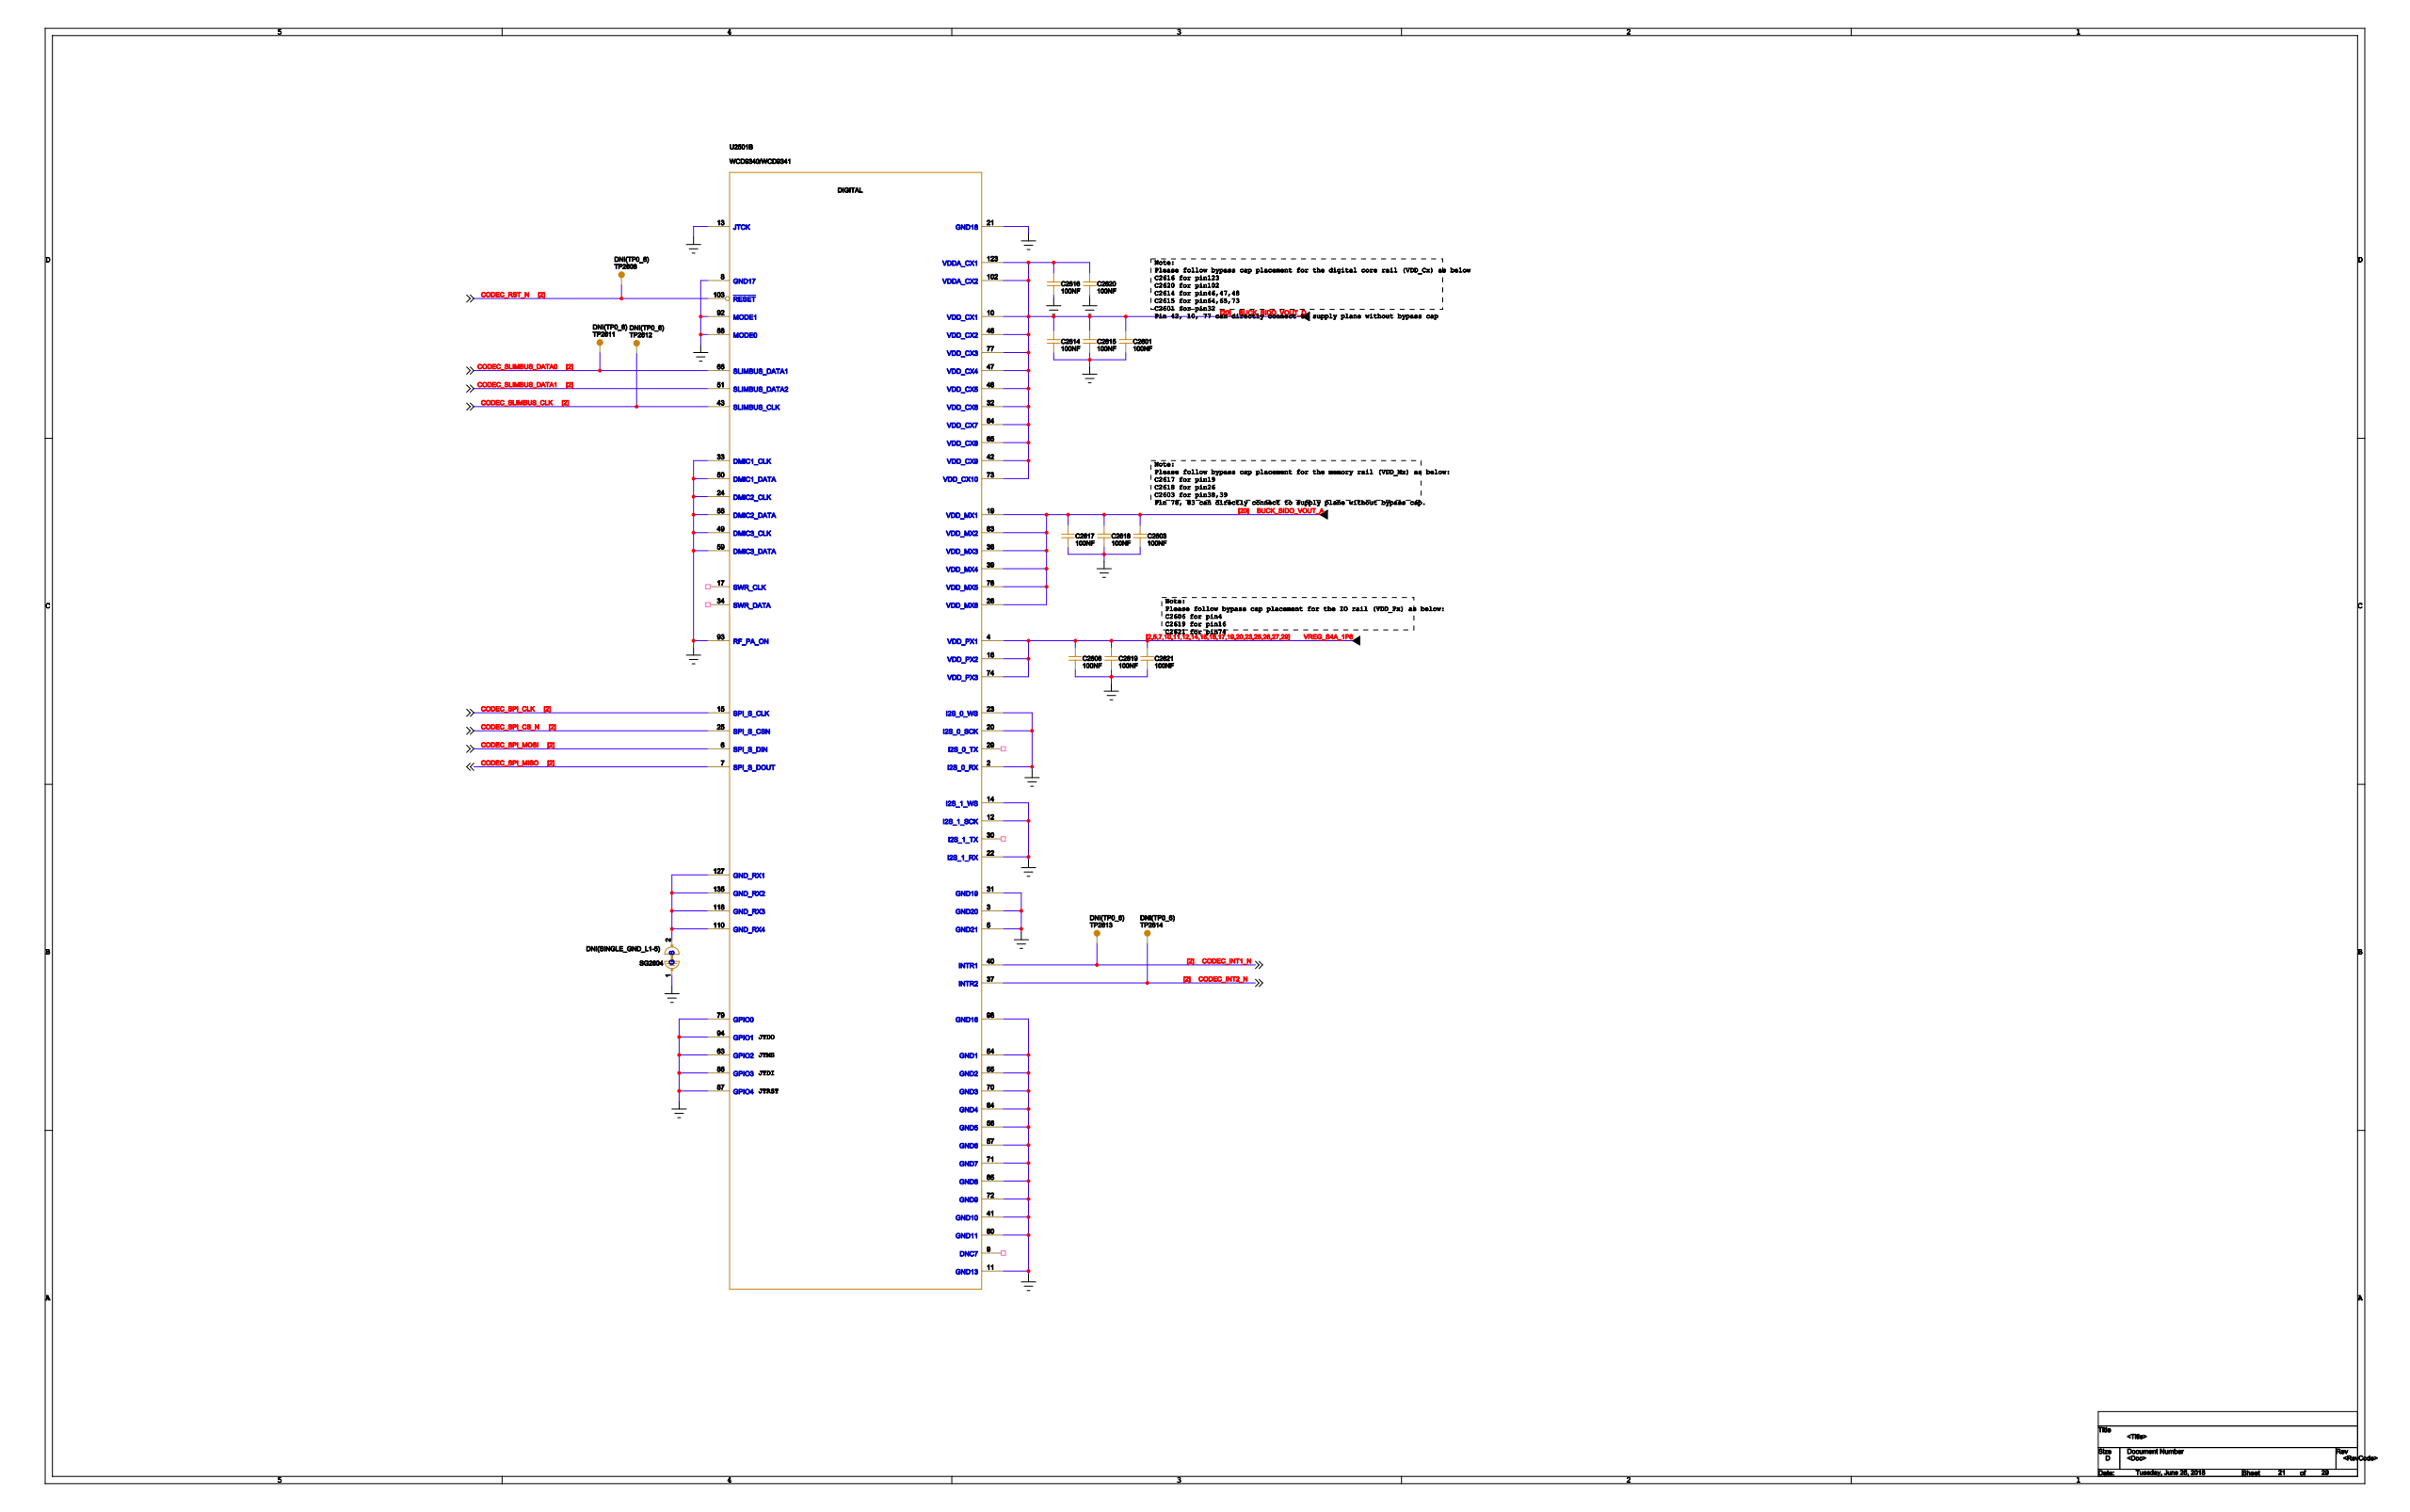Circuit board | Cadence Allegro | 802 parts | 566 nets | one sheet of the schematic
Parts on this sheet (reference | value | footprint):
C2601 | 100NF | C0201
C2603 | 100NF | C0201
C2606 | 100NF | C0201
C2614 | 100NF | C0201
C2615 | 100NF | C0201
C2616 | 100NF | C0201
C2617 | 100NF | C0201
C2618 | 100NF | C0201
C2619 | 100NF | C0201
C2620 | 100NF | C0201
C2621 | 100NF | C0201
SG2604 | DNI(SINGLE_GND_L1-5) | GND_L1-5
TP2608 | DNI(TP0_6) | TP_C0P6
TP2611 | DNI(TP0_6) | TP_C0P6
TP2612 | DNI(TP0_6) | TP_C0P6
TP2613 | DNI(TP0_6) | TP_C0P6
TP2614 | DNI(TP0_6) | TP_C0P6
U2501 | WCD9340/WCD9341 | WLPSP154_4P93X4P30X0P65_0P35
Nets of these parts (net: part-pin ...):
GND: C2601-2 C2603-2 C2606-2 C2614-2 C2615-2 C2616-2 C2617-2 C2618-2 C2619-2 C2620-2 C2621-2 SG2604-1 U2501-2 U2501-3 U2501-5 U2501-8 U2501-11 U2501-12 U2501-13 U2501-14 U2501-20 U2501-21 U2501-22 U2501-23 U2501-24 U2501-31 U2501-33 U2501-41 U2501-49 U2501-50 U2501-54 U2501-55 U2501-56 U2501-57 U2501-58 U2501-59 U2501-63 U2501-70 U2501-71 U2501-72 U2501-79 U2501-80 U2501-84 U2501-85 U2501-86 U2501-87 U2501-88 U2501-92 U2501-93 U2501-94 U2501-98
VREG_S4A_1P8: C2606-1 C2619-1 C2621-1 U2501-4 U2501-16 U2501-74
BUCK_SIDO_VOUT_A: C2603-1 C2617-1 C2618-1 U2501-19 U2501-26 U2501-38 U2501-39 U2501-78 U2501-83
BUCK_SIDO_VOUT_D: C2601-1 C2614-1 C2615-1 C2616-1 C2620-1 U2501-10 U2501-32 U2501-42 U2501-46 U2501-47 U2501-48 U2501-64 U2501-65 U2501-73 U2501-77 U2501-102 U2501-123
N290418: SG2604-2 U2501-110 U2501-118 U2501-127 U2501-135
CODEC_RST_N: TP2608-1 U2501-103
CODEC_SLIMBUS_DATA0: TP2611-1 U2501-66
CODEC_SLIMBUS_CLK: TP2612-1 U2501-43
CODEC_INT1_N: TP2613-1 U2501-40
CODEC_INT2_N: TP2614-1 U2501-37
CODEC_SPI_MISO: U2501-7
CODEC_SPI_MOSI: U2501-6
CODEC_SPI_CLK: U2501-15
CODEC_SPI_CS_N: U2501-25
CODEC_SLIMBUS_DATA1: U2501-51